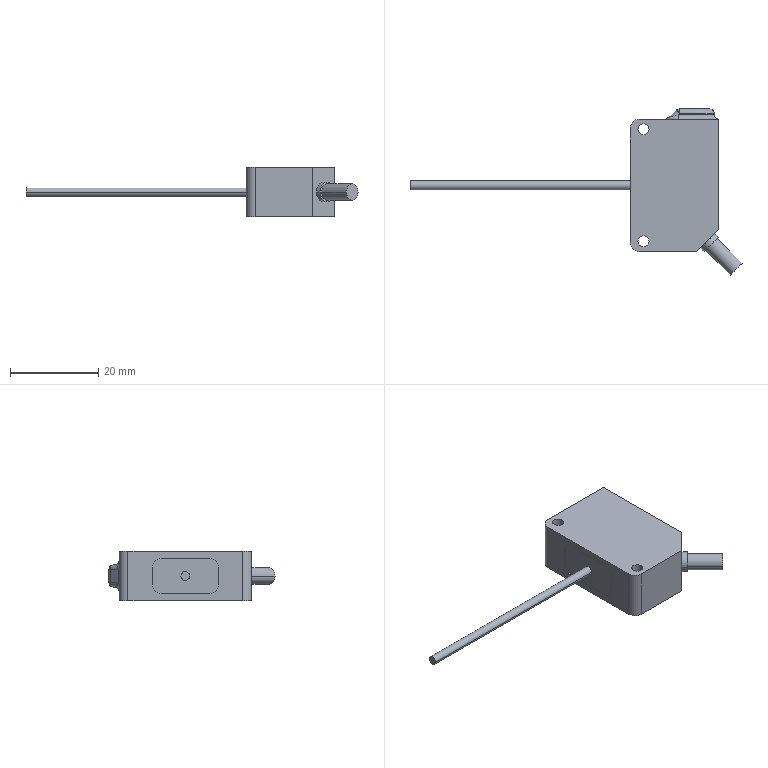Part | SolidWorks | features BaseBody 1 | 1 solid | 64 faces | box 75.214 x 37.614 x 11.2 mm | volume 6810 mm3 | plane 34 | cylinder 26 | sphere 2 | spline 2 | commonest cylinder face diameters 2 x12 4 x6 2.5 x4 3.7 x2 4.5 x2